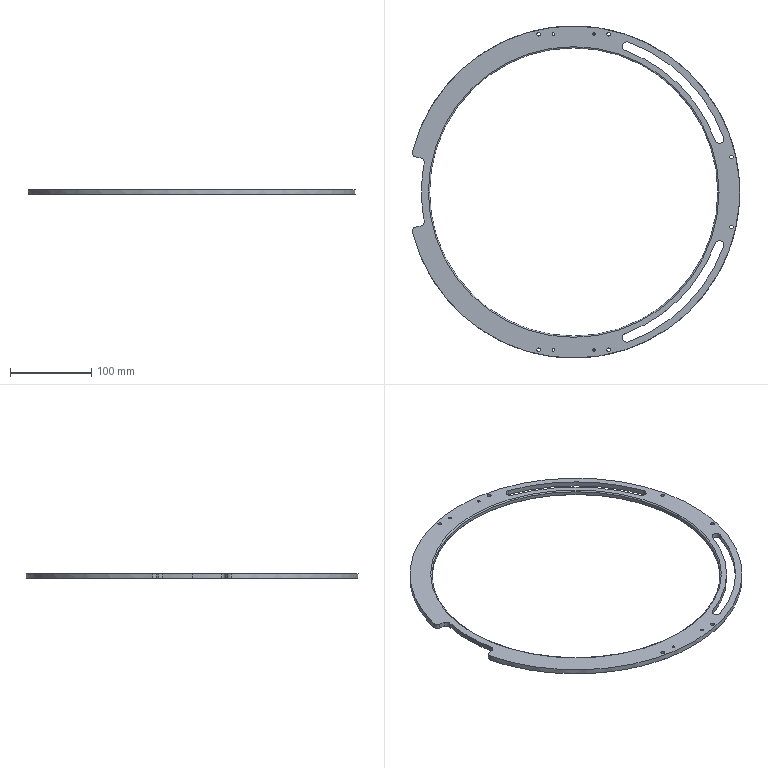Part | NX | features BREP 1 | 1 solid | 61 faces | box 403.128 x 409 x 6 mm | volume 160648 mm3 | cylinder 41 | cone 14 | plane 4 | torus 2 | commonest cylinder face diameters 4.5 x12 3.2 x8 10 x6 11 x6 355 x2 371 x2